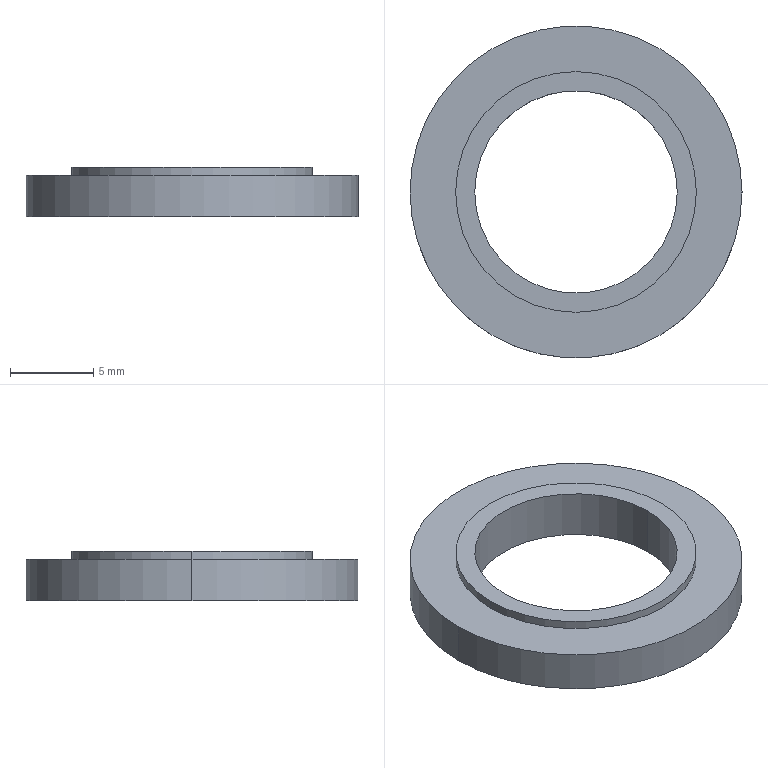Part | SolidWorks | features Revolution 1 | 1 solid | 9 faces | box 20 x 20 x 3 mm | volume 517.267 mm3 | cylinder 6 | plane 3 | commonest cylinder face diameters 12.2 x2 14.5 x2 20 x2
STEP:
#1=CARTESIAN_POINT('',(-7.25,0.,1.5));
#2=VERTEX_POINT('',#1);
#3=CARTESIAN_POINT('',(7.25,0.,1.5));
#4=VERTEX_POINT('',#3);
#5=CARTESIAN_POINT('',(0.,0.,1.5));
#6=DIRECTION('',(0.,0.,-1.));
#7=DIRECTION('',(-1.,0.,0.));
#8=AXIS2_PLACEMENT_3D('',#5,#6,#7);
#9=CIRCLE('',#8,7.25);
#10=EDGE_CURVE('',#2,#4,#9,.T.);
#11=ORIENTED_EDGE('',*,*,#10,.T.);
#12=CARTESIAN_POINT('',(7.25,0.,1.));
#13=VERTEX_POINT('',#12);
#14=CARTESIAN_POINT('',(7.25,0.,1.5));
#15=DIRECTION('',(0.,0.,-1.));
#16=VECTOR('',#15,1000.);
#17=LINE('',#14,#16);
#18=EDGE_CURVE('',#4,#13,#17,.T.);
#19=ORIENTED_EDGE('',*,*,#18,.T.);
#20=CARTESIAN_POINT('',(-7.25,0.,1.));
#21=VERTEX_POINT('',#20);
#22=CARTESIAN_POINT('',(0.,0.,1.));
#23=DIRECTION('',(0.,0.,-1.));
#24=DIRECTION('',(-1.,0.,0.));
#25=AXIS2_PLACEMENT_3D('',#22,#23,#24);
#26=CIRCLE('',#25,7.25);
#27=EDGE_CURVE('',#21,#13,#26,.T.);
#28=ORIENTED_EDGE('',*,*,#27,.F.);
#29=CARTESIAN_POINT('',(-7.25,0.,1.5));
#30=DIRECTION('',(0.,0.,-1.));
#31=VECTOR('',#30,1000.);
#32=LINE('',#29,#31);
#33=EDGE_CURVE('',#2,#21,#32,.T.);
#34=ORIENTED_EDGE('',*,*,#33,.F.);
#35=EDGE_LOOP('',(#11,#19,#28,#34));
#36=FACE_OUTER_BOUND('',#35,.T.);
#37=CARTESIAN_POINT('',(0.,0.,1.5));
#38=DIRECTION('',(0.,0.,-1.));
#39=DIRECTION('',(-1.,0.,0.));
#40=AXIS2_PLACEMENT_3D('',#37,#38,#39);
#41=CYLINDRICAL_SURFACE('',#40,7.25);
#42=ADVANCED_FACE('',(#36),#41,.T.);
#43=CARTESIAN_POINT('',(-10.,0.,1.));
#44=VERTEX_POINT('',#43);
#45=CARTESIAN_POINT('',(10.,0.,1.));
#46=VERTEX_POINT('',#45);
#47=CARTESIAN_POINT('',(0.,0.,1.));
#48=DIRECTION('',(0.,0.,-1.));
#49=DIRECTION('',(-1.,0.,0.));
#50=AXIS2_PLACEMENT_3D('',#47,#48,#49);
#51=CIRCLE('',#50,10.);
#52=EDGE_CURVE('',#44,#46,#51,.T.);
#53=ORIENTED_EDGE('',*,*,#52,.T.);
#54=CARTESIAN_POINT('',(10.,0.,-1.5));
#55=VERTEX_POINT('',#54);
#56=CARTESIAN_POINT('',(10.,0.,1.5));
#57=DIRECTION('',(0.,0.,-1.));
#58=VECTOR('',#57,1000.);
#59=LINE('',#56,#58);
#60=EDGE_CURVE('',#46,#55,#59,.T.);
#61=ORIENTED_EDGE('',*,*,#60,.T.);
#62=CARTESIAN_POINT('',(-10.,0.,-1.5));
#63=VERTEX_POINT('',#62);
#64=CARTESIAN_POINT('',(0.,0.,-1.5));
#65=DIRECTION('',(0.,0.,-1.));
#66=DIRECTION('',(-1.,0.,0.));
#67=AXIS2_PLACEMENT_3D('',#64,#65,#66);
#68=CIRCLE('',#67,10.);
#69=EDGE_CURVE('',#63,#55,#68,.T.);
#70=ORIENTED_EDGE('',*,*,#69,.F.);
#71=CARTESIAN_POINT('',(-10.,0.,1.5));
#72=DIRECTION('',(0.,0.,-1.));
#73=VECTOR('',#72,1000.);
#74=LINE('',#71,#73);
#75=EDGE_CURVE('',#44,#63,#74,.T.);
#76=ORIENTED_EDGE('',*,*,#75,.F.);
#77=EDGE_LOOP('',(#53,#61,#70,#76));
#78=FACE_OUTER_BOUND('',#77,.T.);
#79=CARTESIAN_POINT('',(0.,0.,1.5));
#80=DIRECTION('',(0.,0.,-1.));
#81=DIRECTION('',(-1.,0.,0.));
#82=AXIS2_PLACEMENT_3D('',#79,#80,#81);
#83=CYLINDRICAL_SURFACE('',#82,10.);
#84=ADVANCED_FACE('',(#78),#83,.T.);
#85=CARTESIAN_POINT('',(6.1,0.,1.5));
#86=VERTEX_POINT('',#85);
#87=CARTESIAN_POINT('',(-6.1,0.,1.5));
#88=VERTEX_POINT('',#87);
#89=CARTESIAN_POINT('',(0.,0.,1.5));
#90=DIRECTION('',(0.,0.,-1.));
#91=DIRECTION('',(-1.,0.,0.));
#92=AXIS2_PLACEMENT_3D('',#89,#90,#91);
#93=CIRCLE('',#92,6.1);
#94=EDGE_CURVE('',#86,#88,#93,.T.);
#95=ORIENTED_EDGE('',*,*,#94,.F.);
#96=CARTESIAN_POINT('',(6.1,0.,-1.5));
#97=VERTEX_POINT('',#96);
#98=CARTESIAN_POINT('',(6.1,0.,1.5));
#99=DIRECTION('',(0.,0.,-1.));
#100=VECTOR('',#99,1000.);
#101=LINE('',#98,#100);
#102=EDGE_CURVE('',#86,#97,#101,.T.);
#103=ORIENTED_EDGE('',*,*,#102,.T.);
#104=CARTESIAN_POINT('',(-6.1,0.,-1.5));
#105=VERTEX_POINT('',#104);
#106=CARTESIAN_POINT('',(0.,0.,-1.5));
#107=DIRECTION('',(0.,0.,-1.));
#108=DIRECTION('',(-1.,0.,0.));
#109=AXIS2_PLACEMENT_3D('',#106,#107,#108);
#110=CIRCLE('',#109,6.1);
#111=EDGE_CURVE('',#97,#105,#110,.T.);
#112=ORIENTED_EDGE('',*,*,#111,.T.);
#113=CARTESIAN_POINT('',(-6.1,0.,1.5));
#114=DIRECTION('',(0.,0.,-1.));
#115=VECTOR('',#114,1000.);
#116=LINE('',#113,#115);
#117=EDGE_CURVE('',#88,#105,#116,.T.);
#118=ORIENTED_EDGE('',*,*,#117,.F.);
#119=EDGE_LOOP('',(#95,#103,#112,#118));
#120=FACE_OUTER_BOUND('',#119,.T.);
#121=CARTESIAN_POINT('',(0.,0.,1.5));
#122=DIRECTION('',(0.,0.,-1.));
#123=DIRECTION('',(-1.,0.,0.));
#124=AXIS2_PLACEMENT_3D('',#121,#122,#123);
#125=CYLINDRICAL_SURFACE('',#124,6.1);
#126=ADVANCED_FACE('',(#120),#125,.F.);
#127=CARTESIAN_POINT('',(0.,0.,1.5));
#128=DIRECTION('',(0.,0.,-1.));
#129=DIRECTION('',(-1.,0.,0.));
#130=AXIS2_PLACEMENT_3D('',#127,#128,#129);
#131=CIRCLE('',#130,6.1);
#132=EDGE_CURVE('',#88,#86,#131,.T.);
#133=ORIENTED_EDGE('',*,*,#132,.T.);
#134=ORIENTED_EDGE('',*,*,#94,.T.);
#135=EDGE_LOOP('',(#133,#134));
#136=FACE_BOUND('',#135,.T.);
#137=ORIENTED_EDGE('',*,*,#10,.F.);
#138=CARTESIAN_POINT('',(0.,0.,1.5));
#139=DIRECTION('',(0.,0.,-1.));
#140=DIRECTION('',(-1.,0.,0.));
#141=AXIS2_PLACEMENT_3D('',#138,#139,#140);
#142=CIRCLE('',#141,7.25);
#143=EDGE_CURVE('',#4,#2,#142,.T.);
#144=ORIENTED_EDGE('',*,*,#143,.F.);
#145=EDGE_LOOP('',(#137,#144));
#146=FACE_OUTER_BOUND('',#145,.T.);
#147=CARTESIAN_POINT('',(7.25,0.,1.5));
#148=DIRECTION('',(0.,0.,1.));
#149=DIRECTION('',(1.,0.,0.));
#150=AXIS2_PLACEMENT_3D('',#147,#148,#149);
#151=PLANE('',#150);
#152=ADVANCED_FACE('',(#136,#146),#151,.T.);
#153=ORIENTED_EDGE('',*,*,#102,.F.);
#154=ORIENTED_EDGE('',*,*,#132,.F.);
#155=ORIENTED_EDGE('',*,*,#117,.T.);
#156=CARTESIAN_POINT('',(0.,0.,-1.5));
#157=DIRECTION('',(0.,0.,-1.));
#158=DIRECTION('',(-1.,0.,0.));
#159=AXIS2_PLACEMENT_3D('',#156,#157,#158);
#160=CIRCLE('',#159,6.1);
#161=EDGE_CURVE('',#105,#97,#160,.T.);
#162=ORIENTED_EDGE('',*,*,#161,.T.);
#163=EDGE_LOOP('',(#153,#154,#155,#162));
#164=FACE_OUTER_BOUND('',#163,.T.);
#165=CARTESIAN_POINT('',(0.,0.,1.5));
#166=DIRECTION('',(0.,0.,-1.));
#167=DIRECTION('',(-1.,0.,0.));
#168=AXIS2_PLACEMENT_3D('',#165,#166,#167);
#169=CYLINDRICAL_SURFACE('',#168,6.1);
#170=ADVANCED_FACE('',(#164),#169,.F.);
#171=ORIENTED_EDGE('',*,*,#69,.T.);
#172=CARTESIAN_POINT('',(0.,0.,-1.5));
#173=DIRECTION('',(0.,0.,-1.));
#174=DIRECTION('',(-1.,0.,0.));
#175=AXIS2_PLACEMENT_3D('',#172,#173,#174);
#176=CIRCLE('',#175,10.);
#177=EDGE_CURVE('',#55,#63,#176,.T.);
#178=ORIENTED_EDGE('',*,*,#177,.T.);
#179=EDGE_LOOP('',(#171,#178));
#180=FACE_OUTER_BOUND('',#179,.T.);
#181=ORIENTED_EDGE('',*,*,#161,.F.);
#182=ORIENTED_EDGE('',*,*,#111,.F.);
#183=EDGE_LOOP('',(#181,#182));
#184=FACE_BOUND('',#183,.T.);
#185=CARTESIAN_POINT('',(6.1,0.,-1.5));
#186=DIRECTION('',(0.,0.,-1.));
#187=DIRECTION('',(-1.,0.,0.));
#188=AXIS2_PLACEMENT_3D('',#185,#186,#187);
#189=PLANE('',#188);
#190=ADVANCED_FACE('',(#180,#184),#189,.T.);
#191=ORIENTED_EDGE('',*,*,#60,.F.);
#192=CARTESIAN_POINT('',(0.,0.,1.));
#193=DIRECTION('',(0.,0.,-1.));
#194=DIRECTION('',(-1.,0.,0.));
#195=AXIS2_PLACEMENT_3D('',#192,#193,#194);
#196=CIRCLE('',#195,10.);
#197=EDGE_CURVE('',#46,#44,#196,.T.);
#198=ORIENTED_EDGE('',*,*,#197,.T.);
#199=ORIENTED_EDGE('',*,*,#75,.T.);
#200=ORIENTED_EDGE('',*,*,#177,.F.);
#201=EDGE_LOOP('',(#191,#198,#199,#200));
#202=FACE_OUTER_BOUND('',#201,.T.);
#203=CARTESIAN_POINT('',(0.,0.,1.5));
#204=DIRECTION('',(0.,0.,-1.));
#205=DIRECTION('',(-1.,0.,0.));
#206=AXIS2_PLACEMENT_3D('',#203,#204,#205);
#207=CYLINDRICAL_SURFACE('',#206,10.);
#208=ADVANCED_FACE('',(#202),#207,.T.);
#209=ORIENTED_EDGE('',*,*,#27,.T.);
#210=CARTESIAN_POINT('',(0.,0.,1.));
#211=DIRECTION('',(0.,0.,-1.));
#212=DIRECTION('',(-1.,0.,0.));
#213=AXIS2_PLACEMENT_3D('',#210,#211,#212);
#214=CIRCLE('',#213,7.25);
#215=EDGE_CURVE('',#13,#21,#214,.T.);
#216=ORIENTED_EDGE('',*,*,#215,.T.);
#217=EDGE_LOOP('',(#209,#216));
#218=FACE_BOUND('',#217,.T.);
#219=ORIENTED_EDGE('',*,*,#52,.F.);
#220=ORIENTED_EDGE('',*,*,#197,.F.);
#221=EDGE_LOOP('',(#219,#220));
#222=FACE_OUTER_BOUND('',#221,.T.);
#223=CARTESIAN_POINT('',(10.,0.,1.));
#224=DIRECTION('',(0.,0.,1.));
#225=DIRECTION('',(1.,0.,0.));
#226=AXIS2_PLACEMENT_3D('',#223,#224,#225);
#227=PLANE('',#226);
#228=ADVANCED_FACE('',(#218,#222),#227,.T.);
#229=ORIENTED_EDGE('',*,*,#18,.F.);
#230=ORIENTED_EDGE('',*,*,#143,.T.);
#231=ORIENTED_EDGE('',*,*,#33,.T.);
#232=ORIENTED_EDGE('',*,*,#215,.F.);
#233=EDGE_LOOP('',(#229,#230,#231,#232));
#234=FACE_OUTER_BOUND('',#233,.T.);
#235=CARTESIAN_POINT('',(0.,0.,1.5));
#236=DIRECTION('',(0.,0.,-1.));
#237=DIRECTION('',(-1.,0.,0.));
#238=AXIS2_PLACEMENT_3D('',#235,#236,#237);
#239=CYLINDRICAL_SURFACE('',#238,7.25);
#240=ADVANCED_FACE('',(#234),#239,.T.);
#241=CLOSED_SHELL('',(#42,#84,#126,#152,#170,#190,#208,#228,#240));
#242=MANIFOLD_SOLID_BREP('',#241);
#243=CARTESIAN_POINT('',(0.,0.,0.));
#244=DIRECTION('',(0.,0.,1.));
#245=DIRECTION('',(1.,0.,0.));
#246=AXIS2_PLACEMENT_3D('',#243,#244,#245);
#247=(LENGTH_UNIT()NAMED_UNIT(*)SI_UNIT(.MILLI.,.METRE.));
#248=UNCERTAINTY_MEASURE_WITH_UNIT(LENGTH_MEASURE(0.00001),#247,'','');
#249=(NAMED_UNIT(*)PLANE_ANGLE_UNIT()SI_UNIT($,.RADIAN.));
#250=(NAMED_UNIT(*)SI_UNIT($,.STERADIAN.)SOLID_ANGLE_UNIT());
#251=(GEOMETRIC_REPRESENTATION_CONTEXT(3)GLOBAL_UNCERTAINTY_ASSIGNED_CONTEXT((#248))GLOBAL_UNIT_ASSIGNED_CONTEXT((#247,#249,#250))REPRESENTATION_CONTEXT('',''));
#252=ADVANCED_BREP_SHAPE_REPRESENTATION('',(#242,#246),#251);